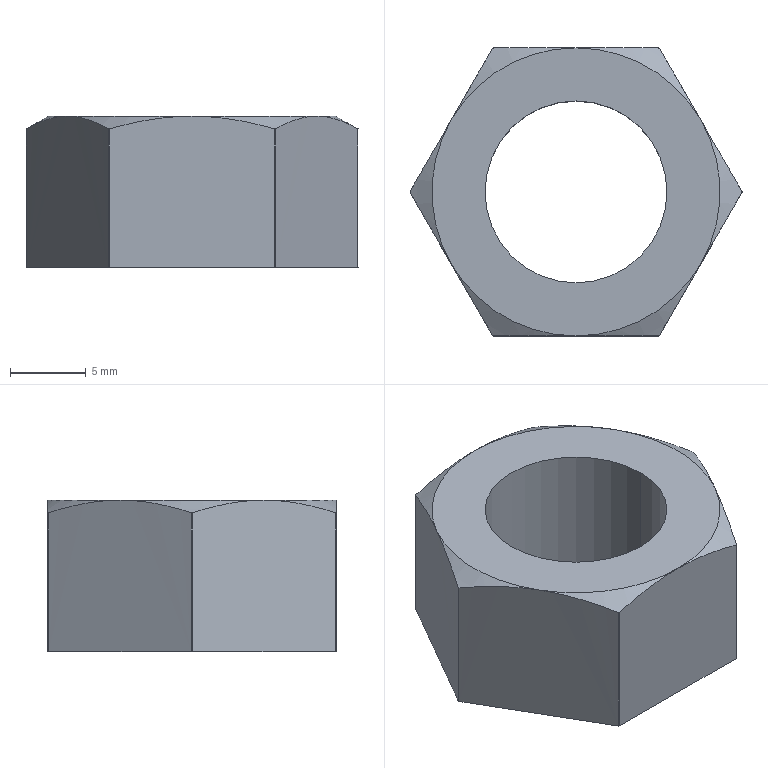Part | STEP file | TNSN20-Y20-F22-Part-11-1 | 1 solid | 22 faces | box 21.9 x 19.004 x 10 mm | volume 1988 mm3 | cylinder 8 | plane 8 | cone 6 | commonest cylinder face diameters 21.9 x6 12 x2
STEP:
#1=CARTESIAN_POINT('',(14083.745,13720.046,15.));
#2=VERTEX_POINT('',#1);
#3=CARTESIAN_POINT('',(14071.745,13720.046,15.));
#4=VERTEX_POINT('',#3);
#5=CARTESIAN_POINT('',(14077.745,13720.046,15.));
#6=DIRECTION('',(0.,0.,-1.));
#7=DIRECTION('',(0.866,-0.5,0.));
#8=AXIS2_PLACEMENT_3D('',#5,#6,#7);
#9=CIRCLE('',#8,6.);
#10=EDGE_CURVE('',#2,#4,#9,.T.);
#11=ORIENTED_EDGE('',*,*,#10,.T.);
#12=CARTESIAN_POINT('',(14071.745,13720.046,25.));
#13=VERTEX_POINT('',#12);
#14=CARTESIAN_POINT('',(14071.745,13720.046,15.));
#15=DIRECTION('',(0.,0.,1.));
#16=VECTOR('',#15,1000.);
#17=LINE('',#14,#16);
#18=EDGE_CURVE('',#4,#13,#17,.T.);
#19=ORIENTED_EDGE('',*,*,#18,.T.);
#20=CARTESIAN_POINT('',(14083.745,13720.046,25.));
#21=VERTEX_POINT('',#20);
#22=CARTESIAN_POINT('',(14077.745,13720.046,25.));
#23=DIRECTION('',(0.,0.,-1.));
#24=DIRECTION('',(0.866,-0.5,0.));
#25=AXIS2_PLACEMENT_3D('',#22,#23,#24);
#26=CIRCLE('',#25,6.);
#27=EDGE_CURVE('',#21,#13,#26,.T.);
#28=ORIENTED_EDGE('',*,*,#27,.F.);
#29=CARTESIAN_POINT('',(14083.745,13720.046,15.));
#30=DIRECTION('',(0.,0.,1.));
#31=VECTOR('',#30,1000.);
#32=LINE('',#29,#31);
#33=EDGE_CURVE('',#2,#21,#32,.T.);
#34=ORIENTED_EDGE('',*,*,#33,.F.);
#35=EDGE_LOOP('',(#11,#19,#28,#34));
#36=FACE_OUTER_BOUND('',#35,.T.);
#37=CARTESIAN_POINT('',(14077.745,13720.046,15.));
#38=DIRECTION('',(0.,0.,1.));
#39=DIRECTION('',(1.,0.,0.));
#40=AXIS2_PLACEMENT_3D('',#37,#38,#39);
#41=CYLINDRICAL_SURFACE('',#40,6.);
#42=ADVANCED_FACE('',(#36),#41,.F.);
#43=CARTESIAN_POINT('',(14072.24,13729.512,24.163));
#44=VERTEX_POINT('',#43);
#45=CARTESIAN_POINT('',(14072.3,13729.546,24.163));
#46=VERTEX_POINT('',#45);
#47=CARTESIAN_POINT('',(14077.745,13720.046,24.163));
#48=DIRECTION('',(0.,0.,-1.));
#49=DIRECTION('',(-0.5027,0.8645,0.));
#50=AXIS2_PLACEMENT_3D('',#47,#48,#49);
#51=CIRCLE('',#50,10.95);
#52=EDGE_CURVE('',#44,#46,#51,.T.);
#53=ORIENTED_EDGE('',*,*,#52,.F.);
#54=CARTESIAN_POINT('',(14069.518,13724.796,25.));
#55=VERTEX_POINT('',#54);
#56=CARTESIAN_POINT('',(14072.24,13729.512,24.163));
#57=CARTESIAN_POINT('',(14072.024,13729.131,24.29));
#58=CARTESIAN_POINT('',(14071.799,13728.744,24.407));
#59=CARTESIAN_POINT('',(14071.347,13727.965,24.612));
#60=CARTESIAN_POINT('',(14071.119,13727.573,24.701));
#61=CARTESIAN_POINT('',(14070.437,13726.391,24.92));
#62=CARTESIAN_POINT('',(14069.986,13725.6,25.002));
#63=CARTESIAN_POINT('',(14069.518,13724.796,25.));
#64=B_SPLINE_CURVE_WITH_KNOTS('',3,(#56,#57,#58,#59,#60,#61,#62,#63),.UNSPECIFIED.,.F.,.F.,(4,2,2,4),(0.,0.25,0.5,1.),.UNSPECIFIED.);
#65=EDGE_CURVE('',#44,#55,#64,.T.);
#66=ORIENTED_EDGE('',*,*,#65,.T.);
#67=CARTESIAN_POINT('',(14077.745,13729.546,25.));
#68=VERTEX_POINT('',#67);
#69=CARTESIAN_POINT('',(14077.745,13720.046,25.));
#70=DIRECTION('',(0.,0.,-1.));
#71=DIRECTION('',(-0.866,0.5,0.));
#72=AXIS2_PLACEMENT_3D('',#69,#70,#71);
#73=CIRCLE('',#72,9.5);
#74=EDGE_CURVE('',#55,#68,#73,.T.);
#75=ORIENTED_EDGE('',*,*,#74,.T.);
#76=CARTESIAN_POINT('',(14077.745,13729.546,25.));
#77=CARTESIAN_POINT('',(14076.815,13729.543,25.002));
#78=CARTESIAN_POINT('',(14075.904,13729.548,24.92));
#79=CARTESIAN_POINT('',(14074.54,13729.548,24.701));
#80=CARTESIAN_POINT('',(14074.086,13729.547,24.612));
#81=CARTESIAN_POINT('',(14073.185,13729.545,24.406));
#82=CARTESIAN_POINT('',(14072.738,13729.543,24.29));
#83=CARTESIAN_POINT('',(14072.3,13729.546,24.163));
#84=B_SPLINE_CURVE_WITH_KNOTS('',3,(#76,#77,#78,#79,#80,#81,#82,#83),.UNSPECIFIED.,.F.,.F.,(4,2,2,4),(0.,0.5,0.75,1.),.UNSPECIFIED.);
#85=EDGE_CURVE('',#68,#46,#84,.T.);
#86=ORIENTED_EDGE('',*,*,#85,.T.);
#87=EDGE_LOOP('',(#53,#66,#75,#86));
#88=FACE_OUTER_BOUND('',#87,.T.);
#89=CARTESIAN_POINT('',(14077.745,13720.046,28.168));
#90=DIRECTION('',(0.,0.,-1.));
#91=DIRECTION('',(0.866,-0.5,0.));
#92=AXIS2_PLACEMENT_3D('',#89,#90,#91);
#93=CONICAL_SURFACE('',#92,4.013,1.047);
#94=ADVANCED_FACE('',(#88),#93,.T.);
#95=CARTESIAN_POINT('',(14069.518,13715.296,25.));
#96=VERTEX_POINT('',#95);
#97=CARTESIAN_POINT('',(14077.745,13720.046,25.));
#98=DIRECTION('',(0.,0.,-1.));
#99=DIRECTION('',(-0.866,-0.5,0.));
#100=AXIS2_PLACEMENT_3D('',#97,#98,#99);
#101=CIRCLE('',#100,9.5);
#102=EDGE_CURVE('',#96,#55,#101,.T.);
#103=ORIENTED_EDGE('',*,*,#102,.T.);
#104=CARTESIAN_POINT('',(14066.795,13720.08,24.163));
#105=VERTEX_POINT('',#104);
#106=CARTESIAN_POINT('',(14069.518,13724.796,25.));
#107=CARTESIAN_POINT('',(14069.055,13723.989,25.002));
#108=CARTESIAN_POINT('',(14068.596,13723.203,24.92));
#109=CARTESIAN_POINT('',(14067.914,13722.021,24.701));
#110=CARTESIAN_POINT('',(14067.688,13721.628,24.612));
#111=CARTESIAN_POINT('',(14067.239,13720.846,24.407));
#112=CARTESIAN_POINT('',(14067.017,13720.459,24.29));
#113=CARTESIAN_POINT('',(14066.795,13720.08,24.163));
#114=B_SPLINE_CURVE_WITH_KNOTS('',3,(#106,#107,#108,#109,#110,#111,#112,#113),.UNSPECIFIED.,.F.,.F.,(4,2,2,4),(0.,0.5,0.75,1.),.UNSPECIFIED.);
#115=EDGE_CURVE('',#55,#105,#114,.T.);
#116=ORIENTED_EDGE('',*,*,#115,.T.);
#117=CARTESIAN_POINT('',(14066.795,13720.012,24.163));
#118=VERTEX_POINT('',#117);
#119=CARTESIAN_POINT('',(14077.745,13720.046,24.163));
#120=DIRECTION('',(0.,0.,-1.));
#121=DIRECTION('',(-1.,-0.003117,0.));
#122=AXIS2_PLACEMENT_3D('',#119,#120,#121);
#123=CIRCLE('',#122,10.95);
#124=EDGE_CURVE('',#118,#105,#123,.T.);
#125=ORIENTED_EDGE('',*,*,#124,.F.);
#126=CARTESIAN_POINT('',(14066.795,13720.012,24.163));
#127=CARTESIAN_POINT('',(14067.017,13719.634,24.29));
#128=CARTESIAN_POINT('',(14067.239,13719.246,24.407));
#129=CARTESIAN_POINT('',(14067.688,13718.465,24.612));
#130=CARTESIAN_POINT('',(14067.914,13718.071,24.701));
#131=CARTESIAN_POINT('',(14068.596,13716.89,24.92));
#132=CARTESIAN_POINT('',(14069.055,13716.103,25.002));
#133=CARTESIAN_POINT('',(14069.518,13715.296,25.));
#134=B_SPLINE_CURVE_WITH_KNOTS('',3,(#126,#127,#128,#129,#130,#131,#132,#133),.UNSPECIFIED.,.F.,.F.,(4,2,2,4),(0.,0.25,0.5,1.),.UNSPECIFIED.);
#135=EDGE_CURVE('',#118,#96,#134,.T.);
#136=ORIENTED_EDGE('',*,*,#135,.T.);
#137=EDGE_LOOP('',(#103,#116,#125,#136));
#138=FACE_OUTER_BOUND('',#137,.T.);
#139=CARTESIAN_POINT('',(14077.745,13720.046,28.168));
#140=DIRECTION('',(0.,0.,-1.));
#141=DIRECTION('',(0.866,-0.5,0.));
#142=AXIS2_PLACEMENT_3D('',#139,#140,#141);
#143=CONICAL_SURFACE('',#142,4.013,1.047);
#144=ADVANCED_FACE('',(#138),#143,.T.);
#145=CARTESIAN_POINT('',(14085.972,13715.296,25.));
#146=VERTEX_POINT('',#145);
#147=CARTESIAN_POINT('',(14077.745,13710.546,25.));
#148=VERTEX_POINT('',#147);
#149=CARTESIAN_POINT('',(14077.745,13720.046,25.));
#150=DIRECTION('',(0.,0.,-1.));
#151=DIRECTION('',(0.866,-0.5,0.));
#152=AXIS2_PLACEMENT_3D('',#149,#150,#151);
#153=CIRCLE('',#152,9.5);
#154=EDGE_CURVE('',#146,#148,#153,.T.);
#155=ORIENTED_EDGE('',*,*,#154,.T.);
#156=CARTESIAN_POINT('',(14083.19,13710.546,24.163));
#157=VERTEX_POINT('',#156);
#158=CARTESIAN_POINT('',(14077.745,13710.546,25.));
#159=CARTESIAN_POINT('',(14078.675,13710.549,25.002));
#160=CARTESIAN_POINT('',(14079.586,13710.545,24.92));
#161=CARTESIAN_POINT('',(14080.95,13710.545,24.701));
#162=CARTESIAN_POINT('',(14081.404,13710.546,24.612));
#163=CARTESIAN_POINT('',(14082.305,13710.548,24.406));
#164=CARTESIAN_POINT('',(14082.752,13710.549,24.29));
#165=CARTESIAN_POINT('',(14083.19,13710.546,24.163));
#166=B_SPLINE_CURVE_WITH_KNOTS('',3,(#158,#159,#160,#161,#162,#163,#164,#165),.UNSPECIFIED.,.F.,.F.,(4,2,2,4),(0.,0.5,0.75,1.),.UNSPECIFIED.);
#167=EDGE_CURVE('',#148,#157,#166,.T.);
#168=ORIENTED_EDGE('',*,*,#167,.T.);
#169=CARTESIAN_POINT('',(14083.249,13710.58,24.163));
#170=VERTEX_POINT('',#169);
#171=CARTESIAN_POINT('',(14077.745,13720.046,24.163));
#172=DIRECTION('',(0.,0.,-1.));
#173=DIRECTION('',(0.5027,-0.8645,0.));
#174=AXIS2_PLACEMENT_3D('',#171,#172,#173);
#175=CIRCLE('',#174,10.95);
#176=EDGE_CURVE('',#170,#157,#175,.T.);
#177=ORIENTED_EDGE('',*,*,#176,.F.);
#178=CARTESIAN_POINT('',(14083.249,13710.58,24.163));
#179=CARTESIAN_POINT('',(14083.466,13710.962,24.29));
#180=CARTESIAN_POINT('',(14083.691,13711.348,24.407));
#181=CARTESIAN_POINT('',(14084.143,13712.127,24.612));
#182=CARTESIAN_POINT('',(14084.371,13712.52,24.701));
#183=CARTESIAN_POINT('',(14085.053,13713.701,24.92));
#184=CARTESIAN_POINT('',(14085.504,13714.492,25.002));
#185=CARTESIAN_POINT('',(14085.972,13715.296,25.));
#186=B_SPLINE_CURVE_WITH_KNOTS('',3,(#178,#179,#180,#181,#182,#183,#184,#185),.UNSPECIFIED.,.F.,.F.,(4,2,2,4),(0.,0.25,0.5,1.),.UNSPECIFIED.);
#187=EDGE_CURVE('',#170,#146,#186,.T.);
#188=ORIENTED_EDGE('',*,*,#187,.T.);
#189=EDGE_LOOP('',(#155,#168,#177,#188));
#190=FACE_OUTER_BOUND('',#189,.T.);
#191=CARTESIAN_POINT('',(14077.745,13720.046,28.168));
#192=DIRECTION('',(0.,0.,-1.));
#193=DIRECTION('',(-0.5,0.866,0.));
#194=AXIS2_PLACEMENT_3D('',#191,#192,#193);
#195=CONICAL_SURFACE('',#194,4.013,1.047);
#196=ADVANCED_FACE('',(#190),#195,.T.);
#197=CARTESIAN_POINT('',(14085.972,13724.796,25.));
#198=VERTEX_POINT('',#197);
#199=CARTESIAN_POINT('',(14077.745,13720.046,25.));
#200=DIRECTION('',(0.,0.,-1.));
#201=DIRECTION('',(0.866,0.5,0.));
#202=AXIS2_PLACEMENT_3D('',#199,#200,#201);
#203=CIRCLE('',#202,9.5);
#204=EDGE_CURVE('',#198,#146,#203,.T.);
#205=ORIENTED_EDGE('',*,*,#204,.T.);
#206=CARTESIAN_POINT('',(14088.695,13720.012,24.163));
#207=VERTEX_POINT('',#206);
#208=CARTESIAN_POINT('',(14085.972,13715.296,25.));
#209=CARTESIAN_POINT('',(14086.435,13716.103,25.002));
#210=CARTESIAN_POINT('',(14086.894,13716.89,24.92));
#211=CARTESIAN_POINT('',(14087.576,13718.071,24.701));
#212=CARTESIAN_POINT('',(14087.802,13718.465,24.612));
#213=CARTESIAN_POINT('',(14088.251,13719.246,24.407));
#214=CARTESIAN_POINT('',(14088.473,13719.634,24.29));
#215=CARTESIAN_POINT('',(14088.695,13720.012,24.163));
#216=B_SPLINE_CURVE_WITH_KNOTS('',3,(#208,#209,#210,#211,#212,#213,#214,#215),.UNSPECIFIED.,.F.,.F.,(4,2,2,4),(0.,0.5,0.75,1.),.UNSPECIFIED.);
#217=EDGE_CURVE('',#146,#207,#216,.T.);
#218=ORIENTED_EDGE('',*,*,#217,.T.);
#219=CARTESIAN_POINT('',(14088.695,13720.08,24.163));
#220=VERTEX_POINT('',#219);
#221=CARTESIAN_POINT('',(14077.745,13720.046,24.163));
#222=DIRECTION('',(0.,0.,-1.));
#223=DIRECTION('',(1.,0.003117,0.));
#224=AXIS2_PLACEMENT_3D('',#221,#222,#223);
#225=CIRCLE('',#224,10.95);
#226=EDGE_CURVE('',#220,#207,#225,.T.);
#227=ORIENTED_EDGE('',*,*,#226,.F.);
#228=CARTESIAN_POINT('',(14088.695,13720.08,24.163));
#229=CARTESIAN_POINT('',(14088.473,13720.459,24.29));
#230=CARTESIAN_POINT('',(14088.251,13720.846,24.407));
#231=CARTESIAN_POINT('',(14087.802,13721.628,24.612));
#232=CARTESIAN_POINT('',(14087.576,13722.021,24.701));
#233=CARTESIAN_POINT('',(14086.894,13723.203,24.92));
#234=CARTESIAN_POINT('',(14086.435,13723.989,25.002));
#235=CARTESIAN_POINT('',(14085.972,13724.796,25.));
#236=B_SPLINE_CURVE_WITH_KNOTS('',3,(#228,#229,#230,#231,#232,#233,#234,#235),.UNSPECIFIED.,.F.,.F.,(4,2,2,4),(0.,0.25,0.5,1.),.UNSPECIFIED.);
#237=EDGE_CURVE('',#220,#198,#236,.T.);
#238=ORIENTED_EDGE('',*,*,#237,.T.);
#239=EDGE_LOOP('',(#205,#218,#227,#238));
#240=FACE_OUTER_BOUND('',#239,.T.);
#241=CARTESIAN_POINT('',(14077.745,13720.046,28.168));
#242=DIRECTION('',(0.,0.,-1.));
#243=DIRECTION('',(-1.,-0.008727,0.));
#244=AXIS2_PLACEMENT_3D('',#241,#242,#243);
#245=CONICAL_SURFACE('',#244,4.013,1.047);
#246=ADVANCED_FACE('',(#240),#245,.T.);
#247=CARTESIAN_POINT('',(14077.745,13720.046,25.));
#248=DIRECTION('',(0.,0.,-1.));
#249=DIRECTION('',(0.,1.,0.));
#250=AXIS2_PLACEMENT_3D('',#247,#248,#249);
#251=CIRCLE('',#250,9.5);
#252=EDGE_CURVE('',#68,#198,#251,.T.);
#253=ORIENTED_EDGE('',*,*,#252,.T.);
#254=CARTESIAN_POINT('',(14083.249,13729.512,24.163));
#255=VERTEX_POINT('',#254);
#256=CARTESIAN_POINT('',(14085.972,13724.796,25.));
#257=CARTESIAN_POINT('',(14085.505,13725.6,25.002));
#258=CARTESIAN_POINT('',(14085.053,13726.391,24.92));
#259=CARTESIAN_POINT('',(14084.371,13727.573,24.701));
#260=CARTESIAN_POINT('',(14084.143,13727.965,24.612));
#261=CARTESIAN_POINT('',(14083.691,13728.744,24.406));
#262=CARTESIAN_POINT('',(14083.466,13729.131,24.29));
#263=CARTESIAN_POINT('',(14083.249,13729.512,24.163));
#264=B_SPLINE_CURVE_WITH_KNOTS('',3,(#256,#257,#258,#259,#260,#261,#262,#263),.UNSPECIFIED.,.F.,.F.,(4,2,2,4),(0.,0.5,0.75,1.),.UNSPECIFIED.);
#265=EDGE_CURVE('',#198,#255,#264,.T.);
#266=ORIENTED_EDGE('',*,*,#265,.T.);
#267=CARTESIAN_POINT('',(14083.19,13729.546,24.163));
#268=VERTEX_POINT('',#267);
#269=CARTESIAN_POINT('',(14077.745,13720.046,24.163));
#270=DIRECTION('',(0.,0.,-1.));
#271=DIRECTION('',(0.4973,0.8676,0.));
#272=AXIS2_PLACEMENT_3D('',#269,#270,#271);
#273=CIRCLE('',#272,10.95);
#274=EDGE_CURVE('',#268,#255,#273,.T.);
#275=ORIENTED_EDGE('',*,*,#274,.F.);
#276=CARTESIAN_POINT('',(14083.19,13729.546,24.163));
#277=CARTESIAN_POINT('',(14082.752,13729.543,24.29));
#278=CARTESIAN_POINT('',(14082.305,13729.544,24.407));
#279=CARTESIAN_POINT('',(14081.404,13729.547,24.612));
#280=CARTESIAN_POINT('',(14080.95,13729.548,24.701));
#281=CARTESIAN_POINT('',(14079.586,13729.548,24.92));
#282=CARTESIAN_POINT('',(14078.675,13729.543,25.002));
#283=CARTESIAN_POINT('',(14077.745,13729.546,25.));
#284=B_SPLINE_CURVE_WITH_KNOTS('',3,(#276,#277,#278,#279,#280,#281,#282,#283),.UNSPECIFIED.,.F.,.F.,(4,2,2,4),(0.,0.25,0.5,1.),.UNSPECIFIED.);
#285=EDGE_CURVE('',#268,#68,#284,.T.);
#286=ORIENTED_EDGE('',*,*,#285,.T.);
#287=EDGE_LOOP('',(#253,#266,#275,#286));
#288=FACE_OUTER_BOUND('',#287,.T.);
#289=CARTESIAN_POINT('',(14077.745,13720.046,28.313));
#290=DIRECTION('',(0.,0.,-1.));
#291=DIRECTION('',(0.866,-0.5,0.));
#292=AXIS2_PLACEMENT_3D('',#289,#290,#291);
#293=CONICAL_SURFACE('',#292,3.762,1.047);
#294=ADVANCED_FACE('',(#288),#293,.T.);
#295=ORIENTED_EDGE('',*,*,#124,.T.);
#296=CARTESIAN_POINT('',(14066.795,13720.08,15.));
#297=VERTEX_POINT('',#296);
#298=CARTESIAN_POINT('',(14066.795,13720.08,24.163));
#299=DIRECTION('',(0.,0.,-1.));
#300=VECTOR('',#299,1000.);
#301=LINE('',#298,#300);
#302=EDGE_CURVE('',#105,#297,#301,.T.);
#303=ORIENTED_EDGE('',*,*,#302,.T.);
#304=CARTESIAN_POINT('',(14066.795,13720.012,15.));
#305=VERTEX_POINT('',#304);
#306=CARTESIAN_POINT('',(14077.745,13720.046,15.));
#307=DIRECTION('',(0.,0.,-1.));
#308=DIRECTION('',(-1.,-0.003117,0.));
#309=AXIS2_PLACEMENT_3D('',#306,#307,#308);
#310=CIRCLE('',#309,10.95);
#311=EDGE_CURVE('',#305,#297,#310,.T.);
#312=ORIENTED_EDGE('',*,*,#311,.F.);
#313=CARTESIAN_POINT('',(14066.795,13720.012,24.163));
#314=DIRECTION('',(0.,0.,-1.));
#315=VECTOR('',#314,1000.);
#316=LINE('',#313,#315);
#317=EDGE_CURVE('',#118,#305,#316,.T.);
#318=ORIENTED_EDGE('',*,*,#317,.F.);
#319=EDGE_LOOP('',(#295,#303,#312,#318));
#320=FACE_OUTER_BOUND('',#319,.T.);
#321=CARTESIAN_POINT('',(14077.745,13720.046,19.581));
#322=DIRECTION('',(0.,0.,-1.));
#323=DIRECTION('',(0.866,-0.5,0.));
#324=AXIS2_PLACEMENT_3D('',#321,#322,#323);
#325=CYLINDRICAL_SURFACE('',#324,10.95);
#326=ADVANCED_FACE('',(#320),#325,.T.);
#327=ORIENTED_EDGE('',*,*,#176,.T.);
#328=CARTESIAN_POINT('',(14083.19,13710.546,15.));
#329=VERTEX_POINT('',#328);
#330=CARTESIAN_POINT('',(14083.19,13710.546,24.163));
#331=DIRECTION('',(0.,0.,-1.));
#332=VECTOR('',#331,1000.);
#333=LINE('',#330,#332);
#334=EDGE_CURVE('',#157,#329,#333,.T.);
#335=ORIENTED_EDGE('',*,*,#334,.T.);
#336=CARTESIAN_POINT('',(14083.249,13710.58,15.));
#337=VERTEX_POINT('',#336);
#338=CARTESIAN_POINT('',(14077.745,13720.046,15.));
#339=DIRECTION('',(0.,0.,-1.));
#340=DIRECTION('',(0.5027,-0.8645,0.));
#341=AXIS2_PLACEMENT_3D('',#338,#339,#340);
#342=CIRCLE('',#341,10.95);
#343=EDGE_CURVE('',#337,#329,#342,.T.);
#344=ORIENTED_EDGE('',*,*,#343,.F.);
#345=CARTESIAN_POINT('',(14083.249,13710.58,24.163));
#346=DIRECTION('',(0.,0.,-1.));
#347=VECTOR('',#346,1000.);
#348=LINE('',#345,#347);
#349=EDGE_CURVE('',#170,#337,#348,.T.);
#350=ORIENTED_EDGE('',*,*,#349,.F.);
#351=EDGE_LOOP('',(#327,#335,#344,#350));
#352=FACE_OUTER_BOUND('',#351,.T.);
#353=CARTESIAN_POINT('',(14077.745,13720.046,19.581));
#354=DIRECTION('',(0.,0.,-1.));
#355=DIRECTION('',(0.866,-0.5,0.));
#356=AXIS2_PLACEMENT_3D('',#353,#354,#355);
#357=CYLINDRICAL_SURFACE('',#356,10.95);
#358=ADVANCED_FACE('',(#352),#357,.T.);
#359=ORIENTED_EDGE('',*,*,#226,.T.);
#360=CARTESIAN_POINT('',(14088.695,13720.012,15.));
#361=VERTEX_POINT('',#360);
#362=CARTESIAN_POINT('',(14088.695,13720.012,24.163));
#363=DIRECTION('',(0.,0.,-1.));
#364=VECTOR('',#363,1000.);
#365=LINE('',#362,#364);
#366=EDGE_CURVE('',#207,#361,#365,.T.);
#367=ORIENTED_EDGE('',*,*,#366,.T.);
#368=CARTESIAN_POINT('',(14088.695,13720.08,15.));
#369=VERTEX_POINT('',#368);
#370=CARTESIAN_POINT('',(14077.745,13720.046,15.));
#371=DIRECTION('',(0.,0.,-1.));
#372=DIRECTION('',(1.,0.003117,0.));
#373=AXIS2_PLACEMENT_3D('',#370,#371,#372);
#374=CIRCLE('',#373,10.95);
#375=EDGE_CURVE('',#369,#361,#374,.T.);
#376=ORIENTED_EDGE('',*,*,#375,.F.);
#377=CARTESIAN_POINT('',(14088.695,13720.08,24.163));
#378=DIRECTION('',(0.,0.,-1.));
#379=VECTOR('',#378,1000.);
#380=LINE('',#377,#379);
#381=EDGE_CURVE('',#220,#369,#380,.T.);
#382=ORIENTED_EDGE('',*,*,#381,.F.);
#383=EDGE_LOOP('',(#359,#367,#376,#382));
#384=FACE_OUTER_BOUND('',#383,.T.);
#385=CARTESIAN_POINT('',(14077.745,13720.046,19.581));
#386=DIRECTION('',(0.,0.,-1.));
#387=DIRECTION('',(0.866,-0.5,0.));
#388=AXIS2_PLACEMENT_3D('',#385,#386,#387);
#389=CYLINDRICAL_SURFACE('',#388,10.95);
#390=ADVANCED_FACE('',(#384),#389,.T.);
#391=ORIENTED_EDGE('',*,*,#274,.T.);
#392=CARTESIAN_POINT('',(14083.249,13729.512,15.));
#393=VERTEX_POINT('',#392);
#394=CARTESIAN_POINT('',(14083.249,13729.512,24.163));
#395=DIRECTION('',(0.,0.,-1.));
#396=VECTOR('',#395,1000.);
#397=LINE('',#394,#396);
#398=EDGE_CURVE('',#255,#393,#397,.T.);
#399=ORIENTED_EDGE('',*,*,#398,.T.);
#400=CARTESIAN_POINT('',(14083.19,13729.546,15.));
#401=VERTEX_POINT('',#400);
#402=CARTESIAN_POINT('',(14077.745,13720.046,15.));
#403=DIRECTION('',(0.,0.,-1.));
#404=DIRECTION('',(0.4973,0.8676,0.));
#405=AXIS2_PLACEMENT_3D('',#402,#403,#404);
#406=CIRCLE('',#405,10.95);
#407=EDGE_CURVE('',#401,#393,#406,.T.);
#408=ORIENTED_EDGE('',*,*,#407,.F.);
#409=CARTESIAN_POINT('',(14083.19,13729.546,24.163));
#410=DIRECTION('',(0.,0.,-1.));
#411=VECTOR('',#410,1000.);
#412=LINE('',#409,#411);
#413=EDGE_CURVE('',#268,#401,#412,.T.);
#414=ORIENTED_EDGE('',*,*,#413,.F.);
#415=EDGE_LOOP('',(#391,#399,#408,#414));
#416=FACE_OUTER_BOUND('',#415,.T.);
#417=CARTESIAN_POINT('',(14077.745,13720.046,19.581));
#418=DIRECTION('',(0.,0.,-1.));
#419=DIRECTION('',(0.866,-0.5,0.));
#420=AXIS2_PLACEMENT_3D('',#417,#418,#419);
#421=CYLINDRICAL_SURFACE('',#420,10.95);
#422=ADVANCED_FACE('',(#416),#421,.T.);
#423=CARTESIAN_POINT('',(14072.24,13729.512,15.));
#424=VERTEX_POINT('',#423);
#425=CARTESIAN_POINT('',(14072.3,13729.546,15.));
#426=VERTEX_POINT('',#425);
#427=CARTESIAN_POINT('',(14077.745,13720.046,15.));
#428=DIRECTION('',(0.,0.,-1.));
#429=DIRECTION('',(-0.5027,0.8645,0.));
#430=AXIS2_PLACEMENT_3D('',#427,#428,#429);
#431=CIRCLE('',#430,10.95);
#432=EDGE_CURVE('',#424,#426,#431,.T.);
#433=ORIENTED_EDGE('',*,*,#432,.F.);
#434=CARTESIAN_POINT('',(14072.24,13729.512,24.163));
#435=DIRECTION('',(0.,0.,-1.));
#436=VECTOR('',#435,1000.);
#437=LINE('',#434,#436);
#438=EDGE_CURVE('',#44,#424,#437,.T.);
#439=ORIENTED_EDGE('',*,*,#438,.F.);
#440=ORIENTED_EDGE('',*,*,#52,.T.);
#441=CARTESIAN_POINT('',(14072.3,13729.546,24.163));
#442=DIRECTION('',(0.,0.,-1.));
#443=VECTOR('',#442,1000.);
#444=LINE('',#441,#443);
#445=EDGE_CURVE('',#46,#426,#444,.T.);
#446=ORIENTED_EDGE('',*,*,#445,.T.);
#447=EDGE_LOOP('',(#433,#439,#440,#446));
#448=FACE_OUTER_BOUND('',#447,.T.);
#449=CARTESIAN_POINT('',(14077.745,13720.046,19.581));
#450=DIRECTION('',(0.,0.,-1.));
#451=DIRECTION('',(0.866,-0.5,0.));
#452=AXIS2_PLACEMENT_3D('',#449,#450,#451);
#453=CYLINDRICAL_SURFACE('',#452,10.95);
#454=ADVANCED_FACE('',(#448),#453,.T.);
#455=CARTESIAN_POINT('',(14077.745,13720.046,25.));
#456=DIRECTION('',(0.,0.,-1.));
#457=DIRECTION('',(0.,-1.,0.));
#458=AXIS2_PLACEMENT_3D('',#455,#456,#457);
#459=CIRCLE('',#458,9.5);
#460=EDGE_CURVE('',#148,#96,#459,.T.);
#461=ORIENTED_EDGE('',*,*,#460,.F.);
#462=ORIENTED_EDGE('',*,*,#154,.F.);
#463=ORIENTED_EDGE('',*,*,#204,.F.);
#464=ORIENTED_EDGE('',*,*,#252,.F.);
#465=ORIENTED_EDGE('',*,*,#74,.F.);
#466=ORIENTED_EDGE('',*,*,#102,.F.);
#467=EDGE_LOOP('',(#461,#462,#463,#464,#465,#466));
#468=FACE_OUTER_BOUND('',#467,.T.);
#469=ORIENTED_EDGE('',*,*,#27,.T.);
#470=CARTESIAN_POINT('',(14077.745,13720.046,25.));
#471=DIRECTION('',(0.,0.,-1.));
#472=DIRECTION('',(0.866,-0.5,0.));
#473=AXIS2_PLACEMENT_3D('',#470,#471,#472);
#474=CIRCLE('',#473,6.);
#475=EDGE_CURVE('',#13,#21,#474,.T.);
#476=ORIENTED_EDGE('',*,*,#475,.T.);
#477=EDGE_LOOP('',(#469,#476));
#478=FACE_BOUND('',#477,.T.);
#479=CARTESIAN_POINT('',(14068.23,13752.142,25.));
#480=DIRECTION('',(0.,0.,-1.));
#481=DIRECTION('',(0.866,-0.5,0.));
#482=AXIS2_PLACEMENT_3D('',#479,#480,#481);
#483=PLANE('',#482);
#484=ADVANCED_FACE('',(#468,#478),#483,.F.);
#485=ORIENTED_EDGE('',*,*,#460,.T.);
#486=CARTESIAN_POINT('',(14072.24,13710.58,24.163));
#487=VERTEX_POINT('',#486);
#488=CARTESIAN_POINT('',(14069.518,13715.296,25.));
#489=CARTESIAN_POINT('',(14069.985,13714.492,25.002));
#490=CARTESIAN_POINT('',(14070.436,13713.701,24.92));
#491=CARTESIAN_POINT('',(14071.119,13712.52,24.701));
#492=CARTESIAN_POINT('',(14071.347,13712.127,24.612));
#493=CARTESIAN_POINT('',(14071.799,13711.348,24.406));
#494=CARTESIAN_POINT('',(14072.024,13710.962,24.29));
#495=CARTESIAN_POINT('',(14072.24,13710.58,24.163));
#496=B_SPLINE_CURVE_WITH_KNOTS('',3,(#488,#489,#490,#491,#492,#493,#494,#495),.UNSPECIFIED.,.F.,.F.,(4,2,2,4),(0.,0.5,0.75,1.),.UNSPECIFIED.);
#497=EDGE_CURVE('',#96,#487,#496,.T.);
#498=ORIENTED_EDGE('',*,*,#497,.T.);
#499=CARTESIAN_POINT('',(14072.3,13710.546,24.163));
#500=VERTEX_POINT('',#499);
#501=CARTESIAN_POINT('',(14077.745,13720.046,24.163));
#502=DIRECTION('',(0.,0.,-1.));
#503=DIRECTION('',(-0.4973,-0.8676,0.));
#504=AXIS2_PLACEMENT_3D('',#501,#502,#503);
#505=CIRCLE('',#504,10.95);
#506=EDGE_CURVE('',#500,#487,#505,.T.);
#507=ORIENTED_EDGE('',*,*,#506,.F.);
#508=CARTESIAN_POINT('',(14072.3,13710.546,24.163));
#509=CARTESIAN_POINT('',(14072.738,13710.549,24.29));
#510=CARTESIAN_POINT('',(14073.185,13710.548,24.407));
#511=CARTESIAN_POINT('',(14074.086,13710.546,24.612));
#512=CARTESIAN_POINT('',(14074.54,13710.545,24.701));
#513=CARTESIAN_POINT('',(14075.904,13710.545,24.92));
#514=CARTESIAN_POINT('',(14076.815,13710.549,25.002));
#515=CARTESIAN_POINT('',(14077.745,13710.546,25.));
#516=B_SPLINE_CURVE_WITH_KNOTS('',3,(#508,#509,#510,#511,#512,#513,#514,#515),.UNSPECIFIED.,.F.,.F.,(4,2,2,4),(0.,0.25,0.5,1.),.UNSPECIFIED.);
#517=EDGE_CURVE('',#500,#148,#516,.T.);
#518=ORIENTED_EDGE('',*,*,#517,.T.);
#519=EDGE_LOOP('',(#485,#498,#507,#518));
#520=FACE_OUTER_BOUND('',#519,.T.);
#521=CARTESIAN_POINT('',(14077.745,13720.046,28.313));
#522=DIRECTION('',(0.,0.,-1.));
#523=DIRECTION('',(0.866,-0.5,0.));
#524=AXIS2_PLACEMENT_3D('',#521,#522,#523);
#525=CONICAL_SURFACE('',#524,3.762,1.047);
#526=ADVANCED_FACE('',(#520),#525,.T.);
#527=CARTESIAN_POINT('',(14072.3,13710.546,15.));
#528=VERTEX_POINT('',#527);
#529=CARTESIAN_POINT('',(14072.24,13710.58,15.));
#530=VERTEX_POINT('',#529);
#531=CARTESIAN_POINT('',(14077.745,13720.046,15.));
#532=DIRECTION('',(0.,0.,-1.));
#533=DIRECTION('',(-0.4973,-0.8676,0.));
#534=AXIS2_PLACEMENT_3D('',#531,#532,#533);
#535=CIRCLE('',#534,10.95);
#536=EDGE_CURVE('',#528,#530,#535,.T.);
#537=ORIENTED_EDGE('',*,*,#536,.F.);
#538=CARTESIAN_POINT('',(14072.3,13710.546,24.163));
#539=DIRECTION('',(0.,0.,-1.));
#540=VECTOR('',#539,1000.);
#541=LINE('',#538,#540);
#542=EDGE_CURVE('',#500,#528,#541,.T.);
#543=ORIENTED_EDGE('',*,*,#542,.F.);
#544=ORIENTED_EDGE('',*,*,#506,.T.);
#545=CARTESIAN_POINT('',(14072.24,13710.58,24.163));
#546=DIRECTION('',(0.,0.,-1.));
#547=VECTOR('',#546,1000.);
#548=LINE('',#545,#547);
#549=EDGE_CURVE('',#487,#530,#548,.T.);
#550=ORIENTED_EDGE('',*,*,#549,.T.);
#551=EDGE_LOOP('',(#537,#543,#544,#550));
#552=FACE_OUTER_BOUND('',#551,.T.);
#553=CARTESIAN_POINT('',(14077.745,13720.046,19.581));
#554=DIRECTION('',(0.,0.,-1.));
#555=DIRECTION('',(0.866,-0.5,0.));
#556=AXIS2_PLACEMENT_3D('',#553,#554,#555);
#557=CYLINDRICAL_SURFACE('',#556,10.95);
#558=ADVANCED_FACE('',(#552),#557,.T.);
#559=ORIENTED_EDGE('',*,*,#311,.T.);
#560=CARTESIAN_POINT('',(14066.795,13720.08,15.));
#561=DIRECTION('',(0.5,0.866,0.));
#562=VECTOR('',#561,1000.);
#563=LINE('',#560,#562);
#564=EDGE_CURVE('',#297,#424,#563,.T.);
#565=ORIENTED_EDGE('',*,*,#564,.T.);
#566=ORIENTED_EDGE('',*,*,#432,.T.);
#567=CARTESIAN_POINT('',(14072.3,13729.546,15.));
#568=DIRECTION('',(1.,0.,0.));
#569=VECTOR('',#568,1000.);
#570=LINE('',#567,#569);
#571=EDGE_CURVE('',#426,#401,#570,.T.);
#572=ORIENTED_EDGE('',*,*,#571,.T.);
#573=ORIENTED_EDGE('',*,*,#407,.T.);
#574=CARTESIAN_POINT('',(14083.249,13729.512,15.));
#575=DIRECTION('',(0.5,-0.866,0.));
#576=VECTOR('',#575,1000.);
#577=LINE('',#574,#576);
#578=EDGE_CURVE('',#393,#369,#577,.T.);
#579=ORIENTED_EDGE('',*,*,#578,.T.);
#580=ORIENTED_EDGE('',*,*,#375,.T.);
#581=CARTESIAN_POINT('',(14088.695,13720.012,15.));
#582=DIRECTION('',(-0.5,-0.866,0.));
#583=VECTOR('',#582,1000.);
#584=LINE('',#581,#583);
#585=EDGE_CURVE('',#361,#337,#584,.T.);
#586=ORIENTED_EDGE('',*,*,#585,.T.);
#587=ORIENTED_EDGE('',*,*,#343,.T.);
#588=CARTESIAN_POINT('',(14083.19,13710.546,15.));
#589=DIRECTION('',(-1.,0.,0.));
#590=VECTOR('',#589,1000.);
#591=LINE('',#588,#590);
#592=EDGE_CURVE('',#329,#528,#591,.T.);
#593=ORIENTED_EDGE('',*,*,#592,.T.);
#594=ORIENTED_EDGE('',*,*,#536,.T.);
#595=CARTESIAN_POINT('',(14072.24,13710.58,15.));
#596=DIRECTION('',(-0.5,0.866,0.));
#597=VECTOR('',#596,1000.);
#598=LINE('',#595,#597);
#599=EDGE_CURVE('',#530,#305,#598,.T.);
#600=ORIENTED_EDGE('',*,*,#599,.T.);
#601=EDGE_LOOP('',(#559,#565,#566,#572,#573,#579,#580,#586,#587,#593,#594,#600));
#602=FACE_OUTER_BOUND('',#601,.T.);
#603=ORIENTED_EDGE('',*,*,#10,.F.);
#604=CARTESIAN_POINT('',(14077.745,13720.046,15.));
#605=DIRECTION('',(0.,0.,-1.));
#606=DIRECTION('',(0.866,-0.5,0.));
#607=AXIS2_PLACEMENT_3D('',#604,#605,#606);
#608=CIRCLE('',#607,6.);
#609=EDGE_CURVE('',#4,#2,#608,.T.);
#610=ORIENTED_EDGE('',*,*,#609,.F.);
#611=EDGE_LOOP('',(#603,#610));
#612=FACE_BOUND('',#611,.T.);
#613=CARTESIAN_POINT('',(14108.105,13729.096,15.));
#614=DIRECTION('',(0.,0.,1.));
#615=DIRECTION('',(-0.866,0.5,0.));
#616=AXIS2_PLACEMENT_3D('',#613,#614,#615);
#617=PLANE('',#616);
#618=ADVANCED_FACE('',(#602,#612),#617,.F.);
#619=ORIENTED_EDGE('',*,*,#85,.F.);
#620=ORIENTED_EDGE('',*,*,#285,.F.);
#621=ORIENTED_EDGE('',*,*,#413,.T.);
#622=ORIENTED_EDGE('',*,*,#571,.F.);
#623=ORIENTED_EDGE('',*,*,#445,.F.);
#624=EDGE_LOOP('',(#619,#620,#621,#622,#623));
#625=FACE_OUTER_BOUND('',#624,.T.);
#626=CARTESIAN_POINT('',(14088.834,13729.546,31.089));
#627=DIRECTION('',(0.,-1.,0.));
#628=DIRECTION('',(-1.,0.,0.));
#629=AXIS2_PLACEMENT_3D('',#626,#627,#628);
#630=PLANE('',#629);
#631=ADVANCED_FACE('',(#625),#630,.F.);
#632=ORIENTED_EDGE('',*,*,#265,.F.);
#633=ORIENTED_EDGE('',*,*,#237,.F.);
#634=ORIENTED_EDGE('',*,*,#381,.T.);
#635=ORIENTED_EDGE('',*,*,#578,.F.);
#636=ORIENTED_EDGE('',*,*,#398,.F.);
#637=EDGE_LOOP('',(#632,#633,#634,#635,#636));
#638=FACE_OUTER_BOUND('',#637,.T.);
#639=CARTESIAN_POINT('',(14091.517,13715.193,31.089));
#640=DIRECTION('',(-0.866,-0.5,0.));
#641=DIRECTION('',(-0.5,0.866,0.));
#642=AXIS2_PLACEMENT_3D('',#639,#640,#641);
#643=PLANE('',#642);
#644=ADVANCED_FACE('',(#638),#643,.F.);
#645=ORIENTED_EDGE('',*,*,#217,.F.);
#646=ORIENTED_EDGE('',*,*,#187,.F.);
#647=ORIENTED_EDGE('',*,*,#349,.T.);
#648=ORIENTED_EDGE('',*,*,#585,.F.);
#649=ORIENTED_EDGE('',*,*,#366,.F.);
#650=EDGE_LOOP('',(#645,#646,#647,#648,#649));
#651=FACE_OUTER_BOUND('',#650,.T.);
#652=CARTESIAN_POINT('',(14091.517,13724.9,31.089));
#653=DIRECTION('',(-0.866,0.5,0.));
#654=DIRECTION('',(0.,0.,-1.));
#655=AXIS2_PLACEMENT_3D('',#652,#653,#654);
#656=PLANE('',#655);
#657=ADVANCED_FACE('',(#651),#656,.F.);
#658=ORIENTED_EDGE('',*,*,#167,.F.);
#659=ORIENTED_EDGE('',*,*,#517,.F.);
#660=ORIENTED_EDGE('',*,*,#542,.T.);
#661=ORIENTED_EDGE('',*,*,#592,.F.);
#662=ORIENTED_EDGE('',*,*,#334,.F.);
#663=EDGE_LOOP('',(#658,#659,#660,#661,#662));
#664=FACE_OUTER_BOUND('',#663,.T.);
#665=CARTESIAN_POINT('',(14066.656,13710.546,31.089));
#666=DIRECTION('',(0.,1.,0.));
#667=DIRECTION('',(1.,0.,0.));
#668=AXIS2_PLACEMENT_3D('',#665,#666,#667);
#669=PLANE('',#668);
#670=ADVANCED_FACE('',(#664),#669,.F.);
#671=ORIENTED_EDGE('',*,*,#497,.F.);
#672=ORIENTED_EDGE('',*,*,#135,.F.);
#673=ORIENTED_EDGE('',*,*,#317,.T.);
#674=ORIENTED_EDGE('',*,*,#599,.F.);
#675=ORIENTED_EDGE('',*,*,#549,.F.);
#676=EDGE_LOOP('',(#671,#672,#673,#674,#675));
#677=FACE_OUTER_BOUND('',#676,.T.);
#678=CARTESIAN_POINT('',(14063.973,13724.9,31.089));
#679=DIRECTION('',(0.866,0.5,0.));
#680=DIRECTION('',(0.5,-0.866,0.));
#681=AXIS2_PLACEMENT_3D('',#678,#679,#680);
#682=PLANE('',#681);
#683=ADVANCED_FACE('',(#677),#682,.F.);
#684=ORIENTED_EDGE('',*,*,#115,.F.);
#685=ORIENTED_EDGE('',*,*,#65,.F.);
#686=ORIENTED_EDGE('',*,*,#438,.T.);
#687=ORIENTED_EDGE('',*,*,#564,.F.);
#688=ORIENTED_EDGE('',*,*,#302,.F.);
#689=EDGE_LOOP('',(#684,#685,#686,#687,#688));
#690=FACE_OUTER_BOUND('',#689,.T.);
#691=CARTESIAN_POINT('',(14075.062,13734.4,8.911));
#692=DIRECTION('',(0.866,-0.5,0.));
#693=DIRECTION('',(0.,0.,1.));
#694=AXIS2_PLACEMENT_3D('',#691,#692,#693);
#695=PLANE('',#694);
#696=ADVANCED_FACE('',(#690),#695,.F.);
#697=ORIENTED_EDGE('',*,*,#18,.F.);
#698=ORIENTED_EDGE('',*,*,#609,.T.);
#699=ORIENTED_EDGE('',*,*,#33,.T.);
#700=ORIENTED_EDGE('',*,*,#475,.F.);
#701=EDGE_LOOP('',(#697,#698,#699,#700));
#702=FACE_OUTER_BOUND('',#701,.T.);
#703=CARTESIAN_POINT('',(14077.745,13720.046,15.));
#704=DIRECTION('',(0.,0.,1.));
#705=DIRECTION('',(1.,0.,0.));
#706=AXIS2_PLACEMENT_3D('',#703,#704,#705);
#707=CYLINDRICAL_SURFACE('',#706,6.);
#708=ADVANCED_FACE('',(#702),#707,.F.);
#709=CLOSED_SHELL('',(#42,#94,#144,#196,#246,#294,#326,#358,#390,#422,#454,#484,#526,#558,#618,#631,#644,#657,#670,#683,#696,#708));
#710=MANIFOLD_SOLID_BREP('',#709);
#711=CARTESIAN_POINT('',(0.,0.,0.));
#712=DIRECTION('',(0.,0.,1.));
#713=DIRECTION('',(1.,0.,0.));
#714=AXIS2_PLACEMENT_3D('',#711,#712,#713);
#715=(LENGTH_UNIT()NAMED_UNIT(*)SI_UNIT(.MILLI.,.METRE.));
#716=UNCERTAINTY_MEASURE_WITH_UNIT(LENGTH_MEASURE(0.00001),#715,'','');
#717=(NAMED_UNIT(*)PLANE_ANGLE_UNIT()SI_UNIT($,.RADIAN.));
#718=(NAMED_UNIT(*)SI_UNIT($,.STERADIAN.)SOLID_ANGLE_UNIT());
#719=(GEOMETRIC_REPRESENTATION_CONTEXT(3)GLOBAL_UNCERTAINTY_ASSIGNED_CONTEXT((#716))GLOBAL_UNIT_ASSIGNED_CONTEXT((#715,#717,#718))REPRESENTATION_CONTEXT('',''));
#720=ADVANCED_BREP_SHAPE_REPRESENTATION('',(#710,#714),#719);